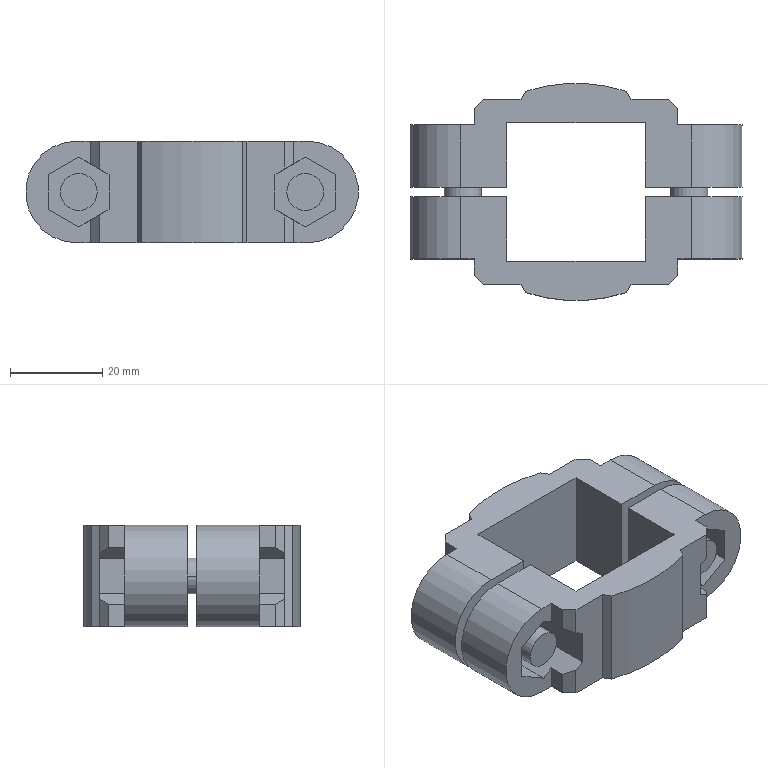Part | STEP file | 29020-30 | 1 solid | 106 faces | box 72 x 47 x 22 mm | volume 32171 mm3 | plane 88 | cylinder 18 | commonest cylinder face diameters 8 x8 13 x4 22 x4 70 x2